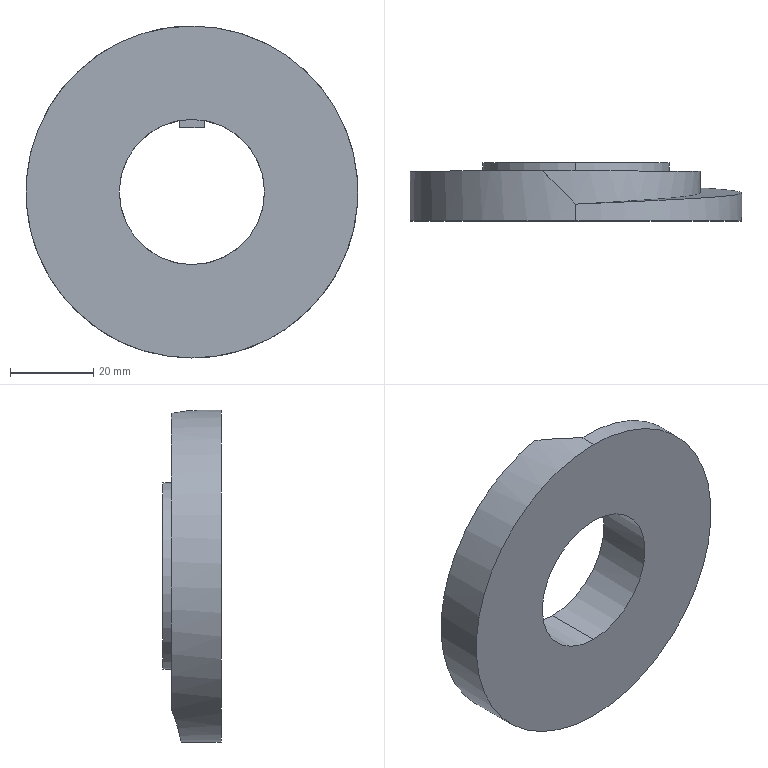Part | SolidWorks | features ICE 3, Chamfer 1, Extrusion 1, Helix 1, SweepCut 1 | 1 solid | 16 faces | box 80 x 14 x 80 mm | volume 43623 mm3 | plane 8 | cylinder 6 | spline 2 | commonest cylinder face diameters 35 x2 45 x2 80 x2